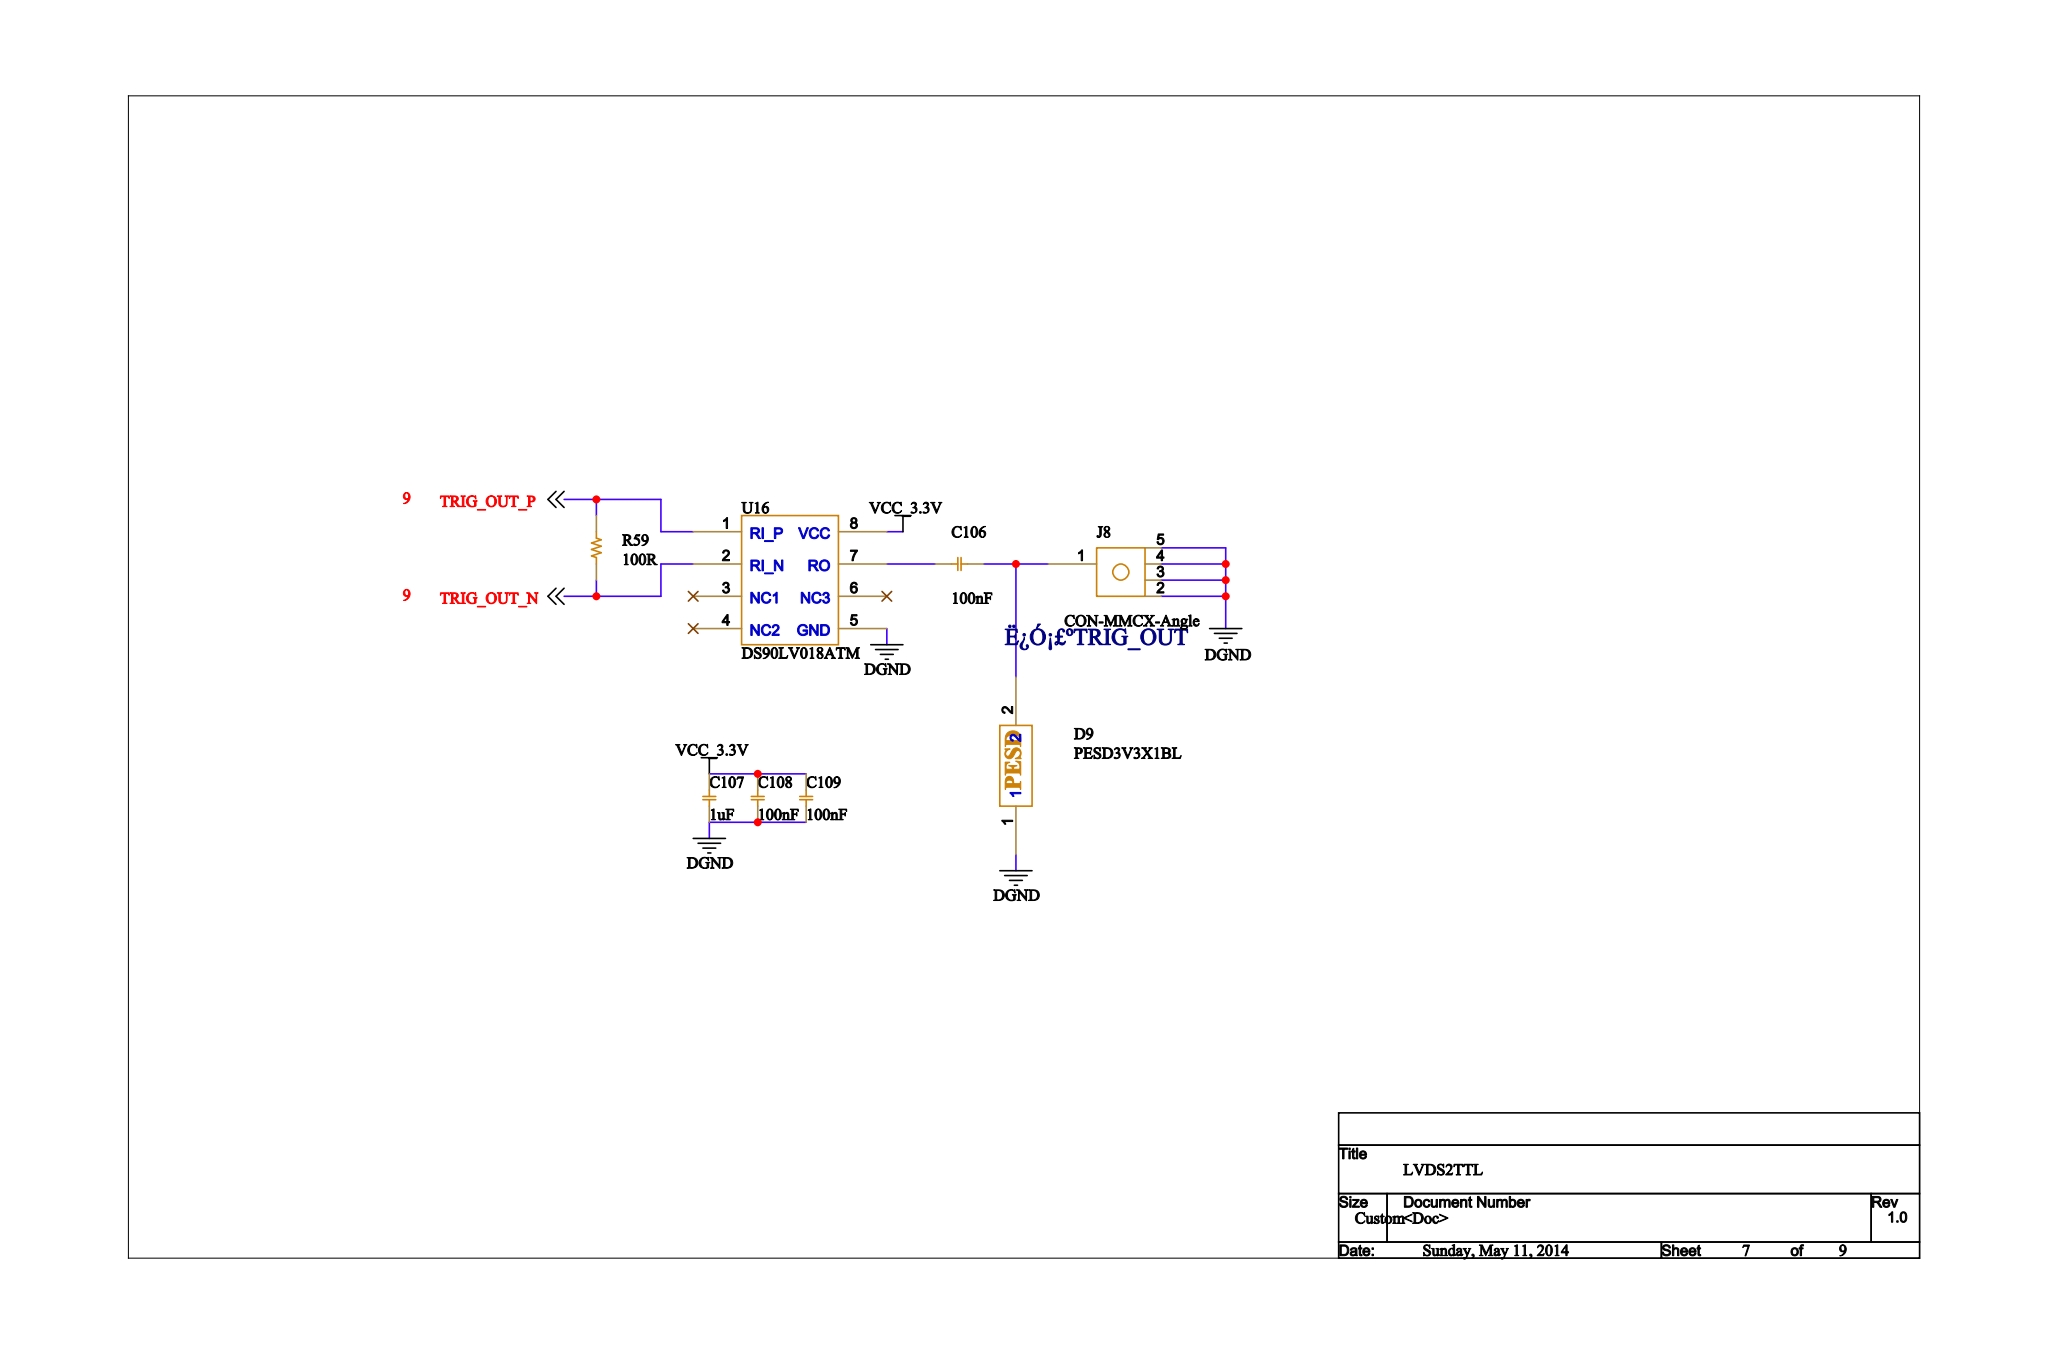Circuit board | Cadence Allegro | 233 parts | 224 nets | one sheet of the schematic
Parts on this sheet (reference | value | footprint):
C106 | 100nF | FPC-0402C
C107 | 1uF | FPC-0402C
C108 | 100nF | FPC-0402C
C109 | 100nF | FPC-0402C
D9 | PESD3V3X1BL | SOD882
J8 | CON-MMCX-Angle | SMA
R59 | 100R | FPC-0603R
U16 | DS90LV018ATM | FPC-SO8-150
Nets of these parts (net: part-pin ...):
DGND: C107-1 C108-1 C109-1 D9-1 J8-2 J8-3 J8-4 J8-5 U16-5
N476277: C106-1 D9-2 J8-1
VCC_3.3V: C107-2 C108-2 C109-2 U16-8
N113378: C106-2 U16-7
TRIG_OUT_N: R59-1 U16-2
TRIG_OUT_P: R59-2 U16-1